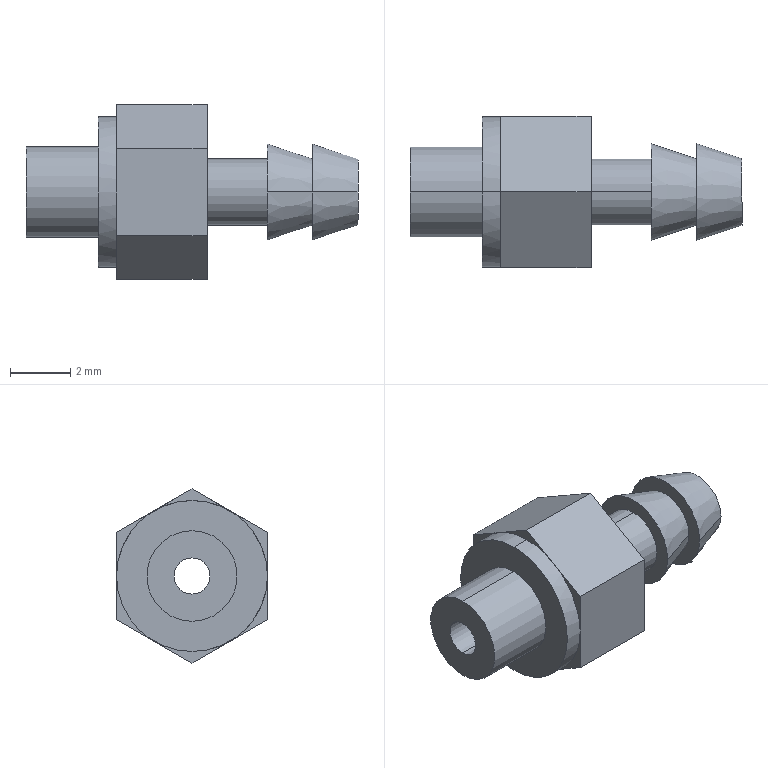Part | SolidWorks | features BaseBody 1 | 1 solid | 29 faces | box 11 x 5 x 5.774 mm | volume 106.233 mm3 | plane 17 | cylinder 8 | cone 4 | commonest cylinder face diameters 1.2 x2 2.2 x2 3 x2 5 x2
STEP:
#1=CARTESIAN_POINT('',(8.6,0.,-0.6));
#2=VERTEX_POINT('',#1);
#3=CARTESIAN_POINT('',(8.6,0.,0.6));
#4=VERTEX_POINT('',#3);
#5=CARTESIAN_POINT('',(8.6,0.,0.));
#6=DIRECTION('',(-1.,0.,0.));
#7=DIRECTION('',(0.,0.,1.));
#8=AXIS2_PLACEMENT_3D('',#5,#6,#7);
#9=CIRCLE('',#8,0.6);
#10=EDGE_CURVE('',#2,#4,#9,.T.);
#11=ORIENTED_EDGE('',*,*,#10,.F.);
#12=CARTESIAN_POINT('',(-2.4,0.,-0.6));
#13=VERTEX_POINT('',#12);
#14=CARTESIAN_POINT('',(-2.675,0.,-0.6));
#15=DIRECTION('',(-1.,0.,0.));
#16=VECTOR('',#15,1000.);
#17=LINE('',#14,#16);
#18=EDGE_CURVE('',#2,#13,#17,.T.);
#19=ORIENTED_EDGE('',*,*,#18,.T.);
#20=CARTESIAN_POINT('',(-2.4,0.,0.6));
#21=VERTEX_POINT('',#20);
#22=CARTESIAN_POINT('',(-2.4,0.,0.));
#23=DIRECTION('',(1.,0.,0.));
#24=DIRECTION('',(0.,0.,1.));
#25=AXIS2_PLACEMENT_3D('',#22,#23,#24);
#26=CIRCLE('',#25,0.6);
#27=EDGE_CURVE('',#21,#13,#26,.T.);
#28=ORIENTED_EDGE('',*,*,#27,.F.);
#29=CARTESIAN_POINT('',(-2.675,0.,0.6));
#30=DIRECTION('',(-1.,0.,0.));
#31=VECTOR('',#30,1000.);
#32=LINE('',#29,#31);
#33=EDGE_CURVE('',#4,#21,#32,.T.);
#34=ORIENTED_EDGE('',*,*,#33,.F.);
#35=EDGE_LOOP('',(#11,#19,#28,#34));
#36=FACE_OUTER_BOUND('',#35,.T.);
#37=CARTESIAN_POINT('',(-2.675,0.,0.));
#38=DIRECTION('',(-1.,0.,0.));
#39=DIRECTION('',(0.,0.,1.));
#40=AXIS2_PLACEMENT_3D('',#37,#38,#39);
#41=CYLINDRICAL_SURFACE('',#40,0.6);
#42=ADVANCED_FACE('',(#36),#41,.F.);
#43=CARTESIAN_POINT('',(8.6,-1.1,0.));
#44=VERTEX_POINT('',#43);
#45=CARTESIAN_POINT('',(8.6,1.1,0.));
#46=VERTEX_POINT('',#45);
#47=CARTESIAN_POINT('',(8.6,0.,0.));
#48=DIRECTION('',(-1.,0.,0.));
#49=DIRECTION('',(0.,-1.,0.));
#50=AXIS2_PLACEMENT_3D('',#47,#48,#49);
#51=CIRCLE('',#50,1.1);
#52=EDGE_CURVE('',#44,#46,#51,.T.);
#53=ORIENTED_EDGE('',*,*,#52,.T.);
#54=CARTESIAN_POINT('',(7.1,1.6,0.));
#55=VERTEX_POINT('',#54);
#56=CARTESIAN_POINT('',(7.1,1.6,0.));
#57=DIRECTION('',(-0.9487,0.3162,0.));
#58=VECTOR('',#57,1000.);
#59=LINE('',#56,#58);
#60=EDGE_CURVE('',#46,#55,#59,.T.);
#61=ORIENTED_EDGE('',*,*,#60,.T.);
#62=CARTESIAN_POINT('',(7.1,-1.6,0.));
#63=VERTEX_POINT('',#62);
#64=CARTESIAN_POINT('',(7.1,0.,0.));
#65=DIRECTION('',(1.,0.,0.));
#66=DIRECTION('',(0.,-1.,0.));
#67=AXIS2_PLACEMENT_3D('',#64,#65,#66);
#68=CIRCLE('',#67,1.6);
#69=EDGE_CURVE('',#55,#63,#68,.T.);
#70=ORIENTED_EDGE('',*,*,#69,.T.);
#71=CARTESIAN_POINT('',(7.1,-1.6,0.));
#72=DIRECTION('',(-0.9487,-0.3162,0.));
#73=VECTOR('',#72,1000.);
#74=LINE('',#71,#73);
#75=EDGE_CURVE('',#44,#63,#74,.T.);
#76=ORIENTED_EDGE('',*,*,#75,.F.);
#77=EDGE_LOOP('',(#53,#61,#70,#76));
#78=FACE_OUTER_BOUND('',#77,.T.);
#79=CARTESIAN_POINT('',(7.1,0.,0.));
#80=DIRECTION('',(-1.,0.,0.));
#81=DIRECTION('',(0.,-1.,0.));
#82=AXIS2_PLACEMENT_3D('',#79,#80,#81);
#83=CONICAL_SURFACE('',#82,1.6,0.3218);
#84=ADVANCED_FACE('',(#78),#83,.T.);
#85=CARTESIAN_POINT('',(-2.4,0.,-1.5));
#86=VERTEX_POINT('',#85);
#87=CARTESIAN_POINT('',(-2.4,0.,1.5));
#88=VERTEX_POINT('',#87);
#89=CARTESIAN_POINT('',(-2.4,0.,0.));
#90=DIRECTION('',(1.,0.,0.));
#91=DIRECTION('',(0.,0.,-1.));
#92=AXIS2_PLACEMENT_3D('',#89,#90,#91);
#93=CIRCLE('',#92,1.5);
#94=EDGE_CURVE('',#86,#88,#93,.T.);
#95=ORIENTED_EDGE('',*,*,#94,.T.);
#96=CARTESIAN_POINT('',(0.,0.,1.5));
#97=VERTEX_POINT('',#96);
#98=CARTESIAN_POINT('',(0.06,0.,1.5));
#99=DIRECTION('',(1.,0.,0.));
#100=VECTOR('',#99,1000.);
#101=LINE('',#98,#100);
#102=EDGE_CURVE('',#88,#97,#101,.T.);
#103=ORIENTED_EDGE('',*,*,#102,.T.);
#104=CARTESIAN_POINT('',(0.,0.,-1.5));
#105=VERTEX_POINT('',#104);
#106=CARTESIAN_POINT('',(0.,0.,0.));
#107=DIRECTION('',(-1.,0.,0.));
#108=DIRECTION('',(0.,0.,-1.));
#109=AXIS2_PLACEMENT_3D('',#106,#107,#108);
#110=CIRCLE('',#109,1.5);
#111=EDGE_CURVE('',#97,#105,#110,.T.);
#112=ORIENTED_EDGE('',*,*,#111,.T.);
#113=CARTESIAN_POINT('',(0.06,0.,-1.5));
#114=DIRECTION('',(1.,0.,0.));
#115=VECTOR('',#114,1000.);
#116=LINE('',#113,#115);
#117=EDGE_CURVE('',#86,#105,#116,.T.);
#118=ORIENTED_EDGE('',*,*,#117,.F.);
#119=EDGE_LOOP('',(#95,#103,#112,#118));
#120=FACE_OUTER_BOUND('',#119,.T.);
#121=CARTESIAN_POINT('',(0.06,0.,0.));
#122=DIRECTION('',(1.,0.,0.));
#123=DIRECTION('',(0.,0.,-1.));
#124=AXIS2_PLACEMENT_3D('',#121,#122,#123);
#125=CYLINDRICAL_SURFACE('',#124,1.5);
#126=ADVANCED_FACE('',(#120),#125,.T.);
#127=CARTESIAN_POINT('',(7.1,-1.1,0.));
#128=VERTEX_POINT('',#127);
#129=CARTESIAN_POINT('',(7.1,1.1,0.));
#130=VERTEX_POINT('',#129);
#131=CARTESIAN_POINT('',(7.1,0.,0.));
#132=DIRECTION('',(-1.,0.,0.));
#133=DIRECTION('',(0.,-1.,0.));
#134=AXIS2_PLACEMENT_3D('',#131,#132,#133);
#135=CIRCLE('',#134,1.1);
#136=EDGE_CURVE('',#128,#130,#135,.T.);
#137=ORIENTED_EDGE('',*,*,#136,.T.);
#138=CARTESIAN_POINT('',(5.6,1.6,0.));
#139=VERTEX_POINT('',#138);
#140=CARTESIAN_POINT('',(5.6,1.6,0.));
#141=DIRECTION('',(-0.9487,0.3162,0.));
#142=VECTOR('',#141,1000.);
#143=LINE('',#140,#142);
#144=EDGE_CURVE('',#130,#139,#143,.T.);
#145=ORIENTED_EDGE('',*,*,#144,.T.);
#146=CARTESIAN_POINT('',(5.6,-1.6,0.));
#147=VERTEX_POINT('',#146);
#148=CARTESIAN_POINT('',(5.6,0.,0.));
#149=DIRECTION('',(1.,0.,0.));
#150=DIRECTION('',(0.,-1.,0.));
#151=AXIS2_PLACEMENT_3D('',#148,#149,#150);
#152=CIRCLE('',#151,1.6);
#153=EDGE_CURVE('',#139,#147,#152,.T.);
#154=ORIENTED_EDGE('',*,*,#153,.T.);
#155=CARTESIAN_POINT('',(5.6,-1.6,0.));
#156=DIRECTION('',(-0.9487,-0.3162,0.));
#157=VECTOR('',#156,1000.);
#158=LINE('',#155,#157);
#159=EDGE_CURVE('',#128,#147,#158,.T.);
#160=ORIENTED_EDGE('',*,*,#159,.F.);
#161=EDGE_LOOP('',(#137,#145,#154,#160));
#162=FACE_OUTER_BOUND('',#161,.T.);
#163=CARTESIAN_POINT('',(5.6,0.,0.));
#164=DIRECTION('',(-1.,0.,0.));
#165=DIRECTION('',(0.,-1.,0.));
#166=AXIS2_PLACEMENT_3D('',#163,#164,#165);
#167=CONICAL_SURFACE('',#166,1.6,0.3218);
#168=ADVANCED_FACE('',(#162),#167,.T.);
#169=CARTESIAN_POINT('',(0.,0.,-2.5));
#170=VERTEX_POINT('',#169);
#171=CARTESIAN_POINT('',(0.,0.,2.5));
#172=VERTEX_POINT('',#171);
#173=CARTESIAN_POINT('',(0.,0.,0.));
#174=DIRECTION('',(1.,0.,0.));
#175=DIRECTION('',(0.,0.,-1.));
#176=AXIS2_PLACEMENT_3D('',#173,#174,#175);
#177=CIRCLE('',#176,2.5);
#178=EDGE_CURVE('',#170,#172,#177,.T.);
#179=ORIENTED_EDGE('',*,*,#178,.T.);
#180=CARTESIAN_POINT('',(0.6,0.,2.5));
#181=VERTEX_POINT('',#180);
#182=CARTESIAN_POINT('',(0.615,0.,2.5));
#183=DIRECTION('',(1.,0.,0.));
#184=VECTOR('',#183,1000.);
#185=LINE('',#182,#184);
#186=EDGE_CURVE('',#172,#181,#185,.T.);
#187=ORIENTED_EDGE('',*,*,#186,.T.);
#188=CARTESIAN_POINT('',(0.6,1.25,2.165));
#189=VERTEX_POINT('',#188);
#190=CARTESIAN_POINT('',(0.6,0.,0.));
#191=DIRECTION('',(-1.,0.,0.));
#192=DIRECTION('',(0.,0.,-1.));
#193=AXIS2_PLACEMENT_3D('',#190,#191,#192);
#194=CIRCLE('',#193,2.5);
#195=EDGE_CURVE('',#181,#189,#194,.T.);
#196=ORIENTED_EDGE('',*,*,#195,.T.);
#197=CARTESIAN_POINT('',(0.6,2.5,0.));
#198=VERTEX_POINT('',#197);
#199=CARTESIAN_POINT('',(0.6,0.,0.));
#200=DIRECTION('',(-1.,0.,0.));
#201=DIRECTION('',(0.,0.,-1.));
#202=AXIS2_PLACEMENT_3D('',#199,#200,#201);
#203=CIRCLE('',#202,2.5);
#204=EDGE_CURVE('',#189,#198,#203,.T.);
#205=ORIENTED_EDGE('',*,*,#204,.T.);
#206=CARTESIAN_POINT('',(0.6,0.,-2.5));
#207=VERTEX_POINT('',#206);
#208=CARTESIAN_POINT('',(0.6,0.,0.));
#209=DIRECTION('',(-1.,0.,0.));
#210=DIRECTION('',(0.,0.,-1.));
#211=AXIS2_PLACEMENT_3D('',#208,#209,#210);
#212=CIRCLE('',#211,2.5);
#213=EDGE_CURVE('',#198,#207,#212,.T.);
#214=ORIENTED_EDGE('',*,*,#213,.T.);
#215=CARTESIAN_POINT('',(0.615,0.,-2.5));
#216=DIRECTION('',(1.,0.,0.));
#217=VECTOR('',#216,1000.);
#218=LINE('',#215,#217);
#219=EDGE_CURVE('',#170,#207,#218,.T.);
#220=ORIENTED_EDGE('',*,*,#219,.F.);
#221=EDGE_LOOP('',(#179,#187,#196,#205,#214,#220));
#222=FACE_OUTER_BOUND('',#221,.T.);
#223=CARTESIAN_POINT('',(0.615,0.,0.));
#224=DIRECTION('',(1.,0.,0.));
#225=DIRECTION('',(0.,0.,-1.));
#226=AXIS2_PLACEMENT_3D('',#223,#224,#225);
#227=CYLINDRICAL_SURFACE('',#226,2.5);
#228=ADVANCED_FACE('',(#222),#227,.T.);
#229=CARTESIAN_POINT('',(3.6,0.,-1.1));
#230=VERTEX_POINT('',#229);
#231=CARTESIAN_POINT('',(3.6,0.,1.1));
#232=VERTEX_POINT('',#231);
#233=CARTESIAN_POINT('',(3.6,0.,0.));
#234=DIRECTION('',(1.,0.,0.));
#235=DIRECTION('',(0.,0.,-1.));
#236=AXIS2_PLACEMENT_3D('',#233,#234,#235);
#237=CIRCLE('',#236,1.1);
#238=EDGE_CURVE('',#230,#232,#237,.T.);
#239=ORIENTED_EDGE('',*,*,#238,.T.);
#240=CARTESIAN_POINT('',(5.6,0.,1.1));
#241=VERTEX_POINT('',#240);
#242=CARTESIAN_POINT('',(5.65,0.,1.1));
#243=DIRECTION('',(1.,0.,0.));
#244=VECTOR('',#243,1000.);
#245=LINE('',#242,#244);
#246=EDGE_CURVE('',#232,#241,#245,.T.);
#247=ORIENTED_EDGE('',*,*,#246,.T.);
#248=CARTESIAN_POINT('',(5.6,0.,-1.1));
#249=VERTEX_POINT('',#248);
#250=CARTESIAN_POINT('',(5.6,0.,0.));
#251=DIRECTION('',(-1.,0.,0.));
#252=DIRECTION('',(0.,0.,-1.));
#253=AXIS2_PLACEMENT_3D('',#250,#251,#252);
#254=CIRCLE('',#253,1.1);
#255=EDGE_CURVE('',#241,#249,#254,.T.);
#256=ORIENTED_EDGE('',*,*,#255,.T.);
#257=CARTESIAN_POINT('',(5.65,0.,-1.1));
#258=DIRECTION('',(1.,0.,0.));
#259=VECTOR('',#258,1000.);
#260=LINE('',#257,#259);
#261=EDGE_CURVE('',#230,#249,#260,.T.);
#262=ORIENTED_EDGE('',*,*,#261,.F.);
#263=EDGE_LOOP('',(#239,#247,#256,#262));
#264=FACE_OUTER_BOUND('',#263,.T.);
#265=CARTESIAN_POINT('',(5.65,0.,0.));
#266=DIRECTION('',(1.,0.,0.));
#267=DIRECTION('',(0.,0.,-1.));
#268=AXIS2_PLACEMENT_3D('',#265,#266,#267);
#269=CYLINDRICAL_SURFACE('',#268,1.1);
#270=ADVANCED_FACE('',(#264),#269,.T.);
#271=ORIENTED_EDGE('',*,*,#18,.F.);
#272=CARTESIAN_POINT('',(8.6,0.,0.));
#273=DIRECTION('',(-1.,0.,0.));
#274=DIRECTION('',(0.,0.,1.));
#275=AXIS2_PLACEMENT_3D('',#272,#273,#274);
#276=CIRCLE('',#275,0.6);
#277=EDGE_CURVE('',#4,#2,#276,.T.);
#278=ORIENTED_EDGE('',*,*,#277,.F.);
#279=ORIENTED_EDGE('',*,*,#33,.T.);
#280=CARTESIAN_POINT('',(-2.4,0.,0.));
#281=DIRECTION('',(1.,0.,0.));
#282=DIRECTION('',(0.,0.,1.));
#283=AXIS2_PLACEMENT_3D('',#280,#281,#282);
#284=CIRCLE('',#283,0.6);
#285=EDGE_CURVE('',#13,#21,#284,.T.);
#286=ORIENTED_EDGE('',*,*,#285,.F.);
#287=EDGE_LOOP('',(#271,#278,#279,#286));
#288=FACE_OUTER_BOUND('',#287,.T.);
#289=CARTESIAN_POINT('',(-2.675,0.,0.));
#290=DIRECTION('',(-1.,0.,0.));
#291=DIRECTION('',(0.,0.,1.));
#292=AXIS2_PLACEMENT_3D('',#289,#290,#291);
#293=CYLINDRICAL_SURFACE('',#292,0.6);
#294=ADVANCED_FACE('',(#288),#293,.F.);
#295=ORIENTED_EDGE('',*,*,#277,.T.);
#296=ORIENTED_EDGE('',*,*,#10,.T.);
#297=EDGE_LOOP('',(#295,#296));
#298=FACE_BOUND('',#297,.T.);
#299=ORIENTED_EDGE('',*,*,#52,.F.);
#300=CARTESIAN_POINT('',(8.6,0.,0.));
#301=DIRECTION('',(-1.,0.,0.));
#302=DIRECTION('',(0.,-1.,0.));
#303=AXIS2_PLACEMENT_3D('',#300,#301,#302);
#304=CIRCLE('',#303,1.1);
#305=EDGE_CURVE('',#46,#44,#304,.T.);
#306=ORIENTED_EDGE('',*,*,#305,.F.);
#307=EDGE_LOOP('',(#299,#306));
#308=FACE_OUTER_BOUND('',#307,.T.);
#309=CARTESIAN_POINT('',(8.6,-1.21,0.000000029));
#310=DIRECTION('',(-1.,0.,0.));
#311=DIRECTION('',(0.,0.,1.));
#312=AXIS2_PLACEMENT_3D('',#309,#310,#311);
#313=PLANE('',#312);
#314=ADVANCED_FACE('',(#298,#308),#313,.F.);
#315=ORIENTED_EDGE('',*,*,#27,.T.);
#316=ORIENTED_EDGE('',*,*,#285,.T.);
#317=EDGE_LOOP('',(#315,#316));
#318=FACE_BOUND('',#317,.T.);
#319=ORIENTED_EDGE('',*,*,#94,.F.);
#320=CARTESIAN_POINT('',(-2.4,0.,0.));
#321=DIRECTION('',(1.,0.,0.));
#322=DIRECTION('',(0.,0.,-1.));
#323=AXIS2_PLACEMENT_3D('',#320,#321,#322);
#324=CIRCLE('',#323,1.5);
#325=EDGE_CURVE('',#88,#86,#324,.T.);
#326=ORIENTED_EDGE('',*,*,#325,.F.);
#327=EDGE_LOOP('',(#319,#326));
#328=FACE_OUTER_BOUND('',#327,.T.);
#329=CARTESIAN_POINT('',(-2.4,-1.65,-0.00000004));
#330=DIRECTION('',(1.,0.,0.));
#331=DIRECTION('',(0.,0.,-1.));
#332=AXIS2_PLACEMENT_3D('',#329,#330,#331);
#333=PLANE('',#332);
#334=ADVANCED_FACE('',(#318,#328),#333,.F.);
#335=ORIENTED_EDGE('',*,*,#60,.F.);
#336=ORIENTED_EDGE('',*,*,#305,.T.);
#337=ORIENTED_EDGE('',*,*,#75,.T.);
#338=CARTESIAN_POINT('',(7.1,0.,0.));
#339=DIRECTION('',(1.,0.,0.));
#340=DIRECTION('',(0.,-1.,0.));
#341=AXIS2_PLACEMENT_3D('',#338,#339,#340);
#342=CIRCLE('',#341,1.6);
#343=EDGE_CURVE('',#63,#55,#342,.T.);
#344=ORIENTED_EDGE('',*,*,#343,.T.);
#345=EDGE_LOOP('',(#335,#336,#337,#344));
#346=FACE_OUTER_BOUND('',#345,.T.);
#347=CARTESIAN_POINT('',(7.1,0.,0.));
#348=DIRECTION('',(-1.,0.,0.));
#349=DIRECTION('',(0.,-1.,0.));
#350=AXIS2_PLACEMENT_3D('',#347,#348,#349);
#351=CONICAL_SURFACE('',#350,1.6,0.3218);
#352=ADVANCED_FACE('',(#346),#351,.T.);
#353=ORIENTED_EDGE('',*,*,#102,.F.);
#354=ORIENTED_EDGE('',*,*,#325,.T.);
#355=ORIENTED_EDGE('',*,*,#117,.T.);
#356=CARTESIAN_POINT('',(0.,0.,0.));
#357=DIRECTION('',(-1.,0.,0.));
#358=DIRECTION('',(0.,0.,-1.));
#359=AXIS2_PLACEMENT_3D('',#356,#357,#358);
#360=CIRCLE('',#359,1.5);
#361=EDGE_CURVE('',#105,#97,#360,.T.);
#362=ORIENTED_EDGE('',*,*,#361,.T.);
#363=EDGE_LOOP('',(#353,#354,#355,#362));
#364=FACE_OUTER_BOUND('',#363,.T.);
#365=CARTESIAN_POINT('',(0.06,0.,0.));
#366=DIRECTION('',(1.,0.,0.));
#367=DIRECTION('',(0.,0.,-1.));
#368=AXIS2_PLACEMENT_3D('',#365,#366,#367);
#369=CYLINDRICAL_SURFACE('',#368,1.5);
#370=ADVANCED_FACE('',(#364),#369,.T.);
#371=ORIENTED_EDGE('',*,*,#136,.F.);
#372=CARTESIAN_POINT('',(7.1,0.,0.));
#373=DIRECTION('',(-1.,0.,0.));
#374=DIRECTION('',(0.,-1.,0.));
#375=AXIS2_PLACEMENT_3D('',#372,#373,#374);
#376=CIRCLE('',#375,1.1);
#377=EDGE_CURVE('',#130,#128,#376,.T.);
#378=ORIENTED_EDGE('',*,*,#377,.F.);
#379=EDGE_LOOP('',(#371,#378));
#380=FACE_BOUND('',#379,.T.);
#381=ORIENTED_EDGE('',*,*,#343,.F.);
#382=ORIENTED_EDGE('',*,*,#69,.F.);
#383=EDGE_LOOP('',(#381,#382));
#384=FACE_OUTER_BOUND('',#383,.T.);
#385=CARTESIAN_POINT('',(7.1,-1.76,-0.000000043));
#386=DIRECTION('',(1.,0.,0.));
#387=DIRECTION('',(0.,0.,-1.));
#388=AXIS2_PLACEMENT_3D('',#385,#386,#387);
#389=PLANE('',#388);
#390=ADVANCED_FACE('',(#380,#384),#389,.F.);
#391=ORIENTED_EDGE('',*,*,#361,.F.);
#392=ORIENTED_EDGE('',*,*,#111,.F.);
#393=EDGE_LOOP('',(#391,#392));
#394=FACE_BOUND('',#393,.T.);
#395=ORIENTED_EDGE('',*,*,#178,.F.);
#396=CARTESIAN_POINT('',(0.,0.,0.));
#397=DIRECTION('',(1.,0.,0.));
#398=DIRECTION('',(0.,0.,-1.));
#399=AXIS2_PLACEMENT_3D('',#396,#397,#398);
#400=CIRCLE('',#399,2.5);
#401=EDGE_CURVE('',#172,#170,#400,.T.);
#402=ORIENTED_EDGE('',*,*,#401,.F.);
#403=EDGE_LOOP('',(#395,#402));
#404=FACE_OUTER_BOUND('',#403,.T.);
#405=CARTESIAN_POINT('',(0.,-2.75,-0.000000067));
#406=DIRECTION('',(1.,0.,0.));
#407=DIRECTION('',(0.,0.,-1.));
#408=AXIS2_PLACEMENT_3D('',#405,#406,#407);
#409=PLANE('',#408);
#410=ADVANCED_FACE('',(#394,#404),#409,.F.);
#411=ORIENTED_EDGE('',*,*,#144,.F.);
#412=ORIENTED_EDGE('',*,*,#377,.T.);
#413=ORIENTED_EDGE('',*,*,#159,.T.);
#414=CARTESIAN_POINT('',(5.6,0.,0.));
#415=DIRECTION('',(1.,0.,0.));
#416=DIRECTION('',(0.,-1.,0.));
#417=AXIS2_PLACEMENT_3D('',#414,#415,#416);
#418=CIRCLE('',#417,1.6);
#419=EDGE_CURVE('',#147,#139,#418,.T.);
#420=ORIENTED_EDGE('',*,*,#419,.T.);
#421=EDGE_LOOP('',(#411,#412,#413,#420));
#422=FACE_OUTER_BOUND('',#421,.T.);
#423=CARTESIAN_POINT('',(5.6,0.,0.));
#424=DIRECTION('',(-1.,0.,0.));
#425=DIRECTION('',(0.,-1.,0.));
#426=AXIS2_PLACEMENT_3D('',#423,#424,#425);
#427=CONICAL_SURFACE('',#426,1.6,0.3218);
#428=ADVANCED_FACE('',(#422),#427,.T.);
#429=ORIENTED_EDGE('',*,*,#186,.F.);
#430=ORIENTED_EDGE('',*,*,#401,.T.);
#431=ORIENTED_EDGE('',*,*,#219,.T.);
#432=CARTESIAN_POINT('',(0.6,-1.241,-2.17));
#433=VERTEX_POINT('',#432);
#434=CARTESIAN_POINT('',(0.6,0.,0.));
#435=DIRECTION('',(-1.,0.,0.));
#436=DIRECTION('',(0.,0.,-1.));
#437=AXIS2_PLACEMENT_3D('',#434,#435,#436);
#438=CIRCLE('',#437,2.5);
#439=EDGE_CURVE('',#207,#433,#438,.T.);
#440=ORIENTED_EDGE('',*,*,#439,.T.);
#441=CARTESIAN_POINT('',(0.6,-1.259,-2.16));
#442=VERTEX_POINT('',#441);
#443=CARTESIAN_POINT('',(0.6,-1.259,-2.16));
#444=CARTESIAN_POINT('',(0.6,-1.253,-2.163));
#445=CARTESIAN_POINT('',(0.6,-1.247,-2.167));
#446=CARTESIAN_POINT('',(0.6,-1.241,-2.17));
#447=B_SPLINE_CURVE_WITH_KNOTS('',3,(#443,#444,#445,#446),.UNSPECIFIED.,.F.,.F.,(4,4),(0.,1.),.UNSPECIFIED.);
#448=EDGE_CURVE('',#442,#433,#447,.T.);
#449=ORIENTED_EDGE('',*,*,#448,.F.);
#450=CARTESIAN_POINT('',(0.6,-2.5,0.));
#451=VERTEX_POINT('',#450);
#452=CARTESIAN_POINT('',(0.6,0.,0.));
#453=DIRECTION('',(-1.,0.,0.));
#454=DIRECTION('',(0.,0.,-1.));
#455=AXIS2_PLACEMENT_3D('',#452,#453,#454);
#456=CIRCLE('',#455,2.5);
#457=EDGE_CURVE('',#442,#451,#456,.T.);
#458=ORIENTED_EDGE('',*,*,#457,.T.);
#459=CARTESIAN_POINT('',(0.6,-1.25,2.165));
#460=VERTEX_POINT('',#459);
#461=CARTESIAN_POINT('',(0.6,0.,0.));
#462=DIRECTION('',(-1.,0.,0.));
#463=DIRECTION('',(0.,0.,-1.));
#464=AXIS2_PLACEMENT_3D('',#461,#462,#463);
#465=CIRCLE('',#464,2.5);
#466=EDGE_CURVE('',#451,#460,#465,.T.);
#467=ORIENTED_EDGE('',*,*,#466,.T.);
#468=CARTESIAN_POINT('',(0.6,0.,0.));
#469=DIRECTION('',(-1.,0.,0.));
#470=DIRECTION('',(0.,0.,-1.));
#471=AXIS2_PLACEMENT_3D('',#468,#469,#470);
#472=CIRCLE('',#471,2.5);
#473=EDGE_CURVE('',#460,#181,#472,.T.);
#474=ORIENTED_EDGE('',*,*,#473,.T.);
#475=EDGE_LOOP('',(#429,#430,#431,#440,#449,#458,#467,#474));
#476=FACE_OUTER_BOUND('',#475,.T.);
#477=CARTESIAN_POINT('',(0.615,0.,0.));
#478=DIRECTION('',(1.,0.,0.));
#479=DIRECTION('',(0.,0.,-1.));
#480=AXIS2_PLACEMENT_3D('',#477,#478,#479);
#481=CYLINDRICAL_SURFACE('',#480,2.5);
#482=ADVANCED_FACE('',(#476),#481,.T.);
#483=CARTESIAN_POINT('',(5.6,0.,0.));
#484=DIRECTION('',(-1.,0.,0.));
#485=DIRECTION('',(0.,0.,-1.));
#486=AXIS2_PLACEMENT_3D('',#483,#484,#485);
#487=CIRCLE('',#486,1.1);
#488=EDGE_CURVE('',#249,#241,#487,.T.);
#489=ORIENTED_EDGE('',*,*,#488,.F.);
#490=ORIENTED_EDGE('',*,*,#255,.F.);
#491=EDGE_LOOP('',(#489,#490));
#492=FACE_BOUND('',#491,.T.);
#493=ORIENTED_EDGE('',*,*,#419,.F.);
#494=ORIENTED_EDGE('',*,*,#153,.F.);
#495=EDGE_LOOP('',(#493,#494));
#496=FACE_OUTER_BOUND('',#495,.T.);
#497=CARTESIAN_POINT('',(5.6,-1.76,-0.000000043));
#498=DIRECTION('',(1.,0.,0.));
#499=DIRECTION('',(0.,0.,-1.));
#500=AXIS2_PLACEMENT_3D('',#497,#498,#499);
#501=PLANE('',#500);
#502=ADVANCED_FACE('',(#492,#496),#501,.F.);
#503=CARTESIAN_POINT('',(0.6,2.5,1.443));
#504=VERTEX_POINT('',#503);
#505=CARTESIAN_POINT('',(0.6,1.25,2.165));
#506=DIRECTION('',(0.,-0.866,0.5));
#507=VECTOR('',#506,1000.);
#508=LINE('',#505,#507);
#509=EDGE_CURVE('',#504,#189,#508,.T.);
#510=ORIENTED_EDGE('',*,*,#509,.F.);
#511=CARTESIAN_POINT('',(0.6,2.5,-0.00002883));
#512=DIRECTION('',(0.,0.,1.));
#513=VECTOR('',#512,1000.);
#514=LINE('',#511,#513);
#515=EDGE_CURVE('',#198,#504,#514,.T.);
#516=ORIENTED_EDGE('',*,*,#515,.F.);
#517=ORIENTED_EDGE('',*,*,#204,.F.);
#518=EDGE_LOOP('',(#510,#516,#517));
#519=FACE_OUTER_BOUND('',#518,.T.);
#520=CARTESIAN_POINT('',(0.6,1.875,-0.1081));
#521=DIRECTION('',(1.,0.,0.));
#522=DIRECTION('',(0.,0.,-1.));
#523=AXIS2_PLACEMENT_3D('',#520,#521,#522);
#524=PLANE('',#523);
#525=ADVANCED_FACE('',(#519),#524,.F.);
#526=CARTESIAN_POINT('',(0.6,0.,2.887));
#527=VERTEX_POINT('',#526);
#528=CARTESIAN_POINT('',(0.6,-1.25,2.165));
#529=DIRECTION('',(0.,-0.866,-0.5));
#530=VECTOR('',#529,1000.);
#531=LINE('',#528,#530);
#532=EDGE_CURVE('',#527,#460,#531,.T.);
#533=ORIENTED_EDGE('',*,*,#532,.F.);
#534=CARTESIAN_POINT('',(0.6,1.25,2.165));
#535=DIRECTION('',(0.,-0.866,0.5));
#536=VECTOR('',#535,1000.);
#537=LINE('',#534,#536);
#538=EDGE_CURVE('',#189,#527,#537,.T.);
#539=ORIENTED_EDGE('',*,*,#538,.F.);
#540=ORIENTED_EDGE('',*,*,#195,.F.);
#541=ORIENTED_EDGE('',*,*,#473,.F.);
#542=EDGE_LOOP('',(#533,#539,#540,#541));
#543=FACE_OUTER_BOUND('',#542,.T.);
#544=CARTESIAN_POINT('',(0.6,-0.000002132,2.129));
#545=DIRECTION('',(1.,0.,0.));
#546=DIRECTION('',(0.,0.,-1.));
#547=AXIS2_PLACEMENT_3D('',#544,#545,#546);
#548=PLANE('',#547);
#549=ADVANCED_FACE('',(#543),#548,.F.);
#550=CARTESIAN_POINT('',(0.6,-2.5,1.443));
#551=VERTEX_POINT('',#550);
#552=CARTESIAN_POINT('',(0.6,-2.5,0.00002383));
#553=DIRECTION('',(0.,0.,-1.));
#554=VECTOR('',#553,1000.);
#555=LINE('',#552,#554);
#556=EDGE_CURVE('',#551,#451,#555,.T.);
#557=ORIENTED_EDGE('',*,*,#556,.F.);
#558=CARTESIAN_POINT('',(0.6,-1.25,2.165));
#559=DIRECTION('',(0.,-0.866,-0.5));
#560=VECTOR('',#559,1000.);
#561=LINE('',#558,#560);
#562=EDGE_CURVE('',#460,#551,#561,.T.);
#563=ORIENTED_EDGE('',*,*,#562,.F.);
#564=ORIENTED_EDGE('',*,*,#466,.F.);
#565=EDGE_LOOP('',(#557,#563,#564));
#566=FACE_OUTER_BOUND('',#565,.T.);
#567=CARTESIAN_POINT('',(0.6,-1.875,-0.1081));
#568=DIRECTION('',(1.,0.,0.));
#569=DIRECTION('',(0.,0.,-1.));
#570=AXIS2_PLACEMENT_3D('',#567,#568,#569);
#571=PLANE('',#570);
#572=ADVANCED_FACE('',(#566),#571,.F.);
#573=CARTESIAN_POINT('',(0.6,-2.5,-1.443));
#574=VERTEX_POINT('',#573);
#575=CARTESIAN_POINT('',(0.6,-1.25,-2.165));
#576=DIRECTION('',(0.,0.866,-0.5));
#577=VECTOR('',#576,1000.);
#578=LINE('',#575,#577);
#579=EDGE_CURVE('',#574,#442,#578,.T.);
#580=ORIENTED_EDGE('',*,*,#579,.F.);
#581=CARTESIAN_POINT('',(0.6,-2.5,0.00002383));
#582=DIRECTION('',(0.,0.,-1.));
#583=VECTOR('',#582,1000.);
#584=LINE('',#581,#583);
#585=EDGE_CURVE('',#451,#574,#584,.T.);
#586=ORIENTED_EDGE('',*,*,#585,.F.);
#587=ORIENTED_EDGE('',*,*,#457,.F.);
#588=EDGE_LOOP('',(#580,#586,#587));
#589=FACE_OUTER_BOUND('',#588,.T.);
#590=CARTESIAN_POINT('',(0.6,-1.88,-2.267));
#591=DIRECTION('',(1.,0.,0.));
#592=DIRECTION('',(0.,0.,-1.));
#593=AXIS2_PLACEMENT_3D('',#590,#591,#592);
#594=PLANE('',#593);
#595=ADVANCED_FACE('',(#589),#594,.F.);
#596=CARTESIAN_POINT('',(0.6,2.5,-1.443));
#597=VERTEX_POINT('',#596);
#598=CARTESIAN_POINT('',(0.6,2.5,-0.00002883));
#599=DIRECTION('',(0.,0.,1.));
#600=VECTOR('',#599,1000.);
#601=LINE('',#598,#600);
#602=EDGE_CURVE('',#597,#198,#601,.T.);
#603=ORIENTED_EDGE('',*,*,#602,.F.);
#604=CARTESIAN_POINT('',(0.6,0.00005,-2.887));
#605=VERTEX_POINT('',#604);
#606=CARTESIAN_POINT('',(0.6,0.00005,-2.887));
#607=DIRECTION('',(0.,0.866,0.5));
#608=VECTOR('',#607,1000.);
#609=LINE('',#606,#608);
#610=EDGE_CURVE('',#605,#597,#609,.T.);
#611=ORIENTED_EDGE('',*,*,#610,.F.);
#612=CARTESIAN_POINT('',(0.6,-1.25,-2.165));
#613=DIRECTION('',(0.,0.866,-0.5));
#614=VECTOR('',#613,1000.);
#615=LINE('',#612,#614);
#616=EDGE_CURVE('',#433,#605,#615,.T.);
#617=ORIENTED_EDGE('',*,*,#616,.F.);
#618=ORIENTED_EDGE('',*,*,#439,.F.);
#619=ORIENTED_EDGE('',*,*,#213,.F.);
#620=EDGE_LOOP('',(#603,#611,#617,#618,#619));
#621=FACE_OUTER_BOUND('',#620,.T.);
#622=CARTESIAN_POINT('',(0.6,0.6297,-3.031));
#623=DIRECTION('',(1.,0.,0.));
#624=DIRECTION('',(0.,0.,-1.));
#625=AXIS2_PLACEMENT_3D('',#622,#623,#624);
#626=PLANE('',#625);
#627=ADVANCED_FACE('',(#621),#626,.F.);
#628=ORIENTED_EDGE('',*,*,#246,.F.);
#629=CARTESIAN_POINT('',(3.6,0.,0.));
#630=DIRECTION('',(1.,0.,0.));
#631=DIRECTION('',(0.,0.,-1.));
#632=AXIS2_PLACEMENT_3D('',#629,#630,#631);
#633=CIRCLE('',#632,1.1);
#634=EDGE_CURVE('',#232,#230,#633,.T.);
#635=ORIENTED_EDGE('',*,*,#634,.T.);
#636=ORIENTED_EDGE('',*,*,#261,.T.);
#637=ORIENTED_EDGE('',*,*,#488,.T.);
#638=EDGE_LOOP('',(#628,#635,#636,#637));
#639=FACE_OUTER_BOUND('',#638,.T.);
#640=CARTESIAN_POINT('',(5.65,0.,0.));
#641=DIRECTION('',(1.,0.,0.));
#642=DIRECTION('',(0.,0.,-1.));
#643=AXIS2_PLACEMENT_3D('',#640,#641,#642);
#644=CYLINDRICAL_SURFACE('',#643,1.1);
#645=ADVANCED_FACE('',(#639),#644,.T.);
#646=CARTESIAN_POINT('',(3.6,2.5,-1.443));
#647=VERTEX_POINT('',#646);
#648=CARTESIAN_POINT('',(3.6,0.00005,-2.887));
#649=VERTEX_POINT('',#648);
#650=CARTESIAN_POINT('',(3.6,1.25,-2.165));
#651=DIRECTION('',(0.,-0.866,-0.5));
#652=VECTOR('',#651,1000.);
#653=LINE('',#650,#652);
#654=EDGE_CURVE('',#647,#649,#653,.T.);
#655=ORIENTED_EDGE('',*,*,#654,.T.);
#656=CARTESIAN_POINT('',(0.4502,0.00005,-2.887));
#657=DIRECTION('',(-1.,0.,0.));
#658=VECTOR('',#657,1000.);
#659=LINE('',#656,#658);
#660=EDGE_CURVE('',#649,#605,#659,.T.);
#661=ORIENTED_EDGE('',*,*,#660,.T.);
#662=ORIENTED_EDGE('',*,*,#610,.T.);
#663=CARTESIAN_POINT('',(0.4502,2.5,-1.443));
#664=DIRECTION('',(1.,0.,0.));
#665=VECTOR('',#664,1000.);
#666=LINE('',#663,#665);
#667=EDGE_CURVE('',#597,#647,#666,.T.);
#668=ORIENTED_EDGE('',*,*,#667,.T.);
#669=EDGE_LOOP('',(#655,#661,#662,#668));
#670=FACE_OUTER_BOUND('',#669,.T.);
#671=CARTESIAN_POINT('',(0.4502,1.25,-2.165));
#672=DIRECTION('',(0.,0.5,-0.866));
#673=DIRECTION('',(0.,0.866,0.5));
#674=AXIS2_PLACEMENT_3D('',#671,#672,#673);
#675=PLANE('',#674);
#676=ADVANCED_FACE('',(#670),#675,.T.);
#677=ORIENTED_EDGE('',*,*,#238,.F.);
#678=ORIENTED_EDGE('',*,*,#634,.F.);
#679=EDGE_LOOP('',(#677,#678));
#680=FACE_BOUND('',#679,.T.);
#681=CARTESIAN_POINT('',(3.6,2.5,1.443));
#682=VERTEX_POINT('',#681);
#683=CARTESIAN_POINT('',(3.6,0.,2.887));
#684=VERTEX_POINT('',#683);
#685=CARTESIAN_POINT('',(3.6,2.5,1.443));
#686=DIRECTION('',(0.,-0.866,0.5));
#687=VECTOR('',#686,1000.);
#688=LINE('',#685,#687);
#689=EDGE_CURVE('',#682,#684,#688,.T.);
#690=ORIENTED_EDGE('',*,*,#689,.T.);
#691=CARTESIAN_POINT('',(3.6,-2.5,1.443));
#692=VERTEX_POINT('',#691);
#693=CARTESIAN_POINT('',(3.6,0.,2.887));
#694=DIRECTION('',(0.,-0.866,-0.5));
#695=VECTOR('',#694,1000.);
#696=LINE('',#693,#695);
#697=EDGE_CURVE('',#684,#692,#696,.T.);
#698=ORIENTED_EDGE('',*,*,#697,.T.);
#699=CARTESIAN_POINT('',(3.6,-2.5,-1.443));
#700=VERTEX_POINT('',#699);
#701=CARTESIAN_POINT('',(3.6,-2.5,-3.175));
#702=DIRECTION('',(0.,0.,-1.));
#703=VECTOR('',#702,1000.);
#704=LINE('',#701,#703);
#705=EDGE_CURVE('',#692,#700,#704,.T.);
#706=ORIENTED_EDGE('',*,*,#705,.T.);
#707=CARTESIAN_POINT('',(3.6,-2.5,-1.443));
#708=DIRECTION('',(0.,0.866,-0.5));
#709=VECTOR('',#708,1000.);
#710=LINE('',#707,#709);
#711=EDGE_CURVE('',#700,#649,#710,.T.);
#712=ORIENTED_EDGE('',*,*,#711,.T.);
#713=ORIENTED_EDGE('',*,*,#654,.F.);
#714=CARTESIAN_POINT('',(3.6,2.5,-3.175));
#715=DIRECTION('',(0.,0.,1.));
#716=VECTOR('',#715,1000.);
#717=LINE('',#714,#716);
#718=EDGE_CURVE('',#647,#682,#717,.T.);
#719=ORIENTED_EDGE('',*,*,#718,.T.);
#720=EDGE_LOOP('',(#690,#698,#706,#712,#713,#719));
#721=FACE_OUTER_BOUND('',#720,.T.);
#722=CARTESIAN_POINT('',(3.6,0.000000067,-3.175));
#723=DIRECTION('',(1.,0.,0.));
#724=DIRECTION('',(0.,0.,-1.));
#725=AXIS2_PLACEMENT_3D('',#722,#723,#724);
#726=PLANE('',#725);
#727=ADVANCED_FACE('',(#680,#721),#726,.T.);
#728=ORIENTED_EDGE('',*,*,#579,.T.);
#729=ORIENTED_EDGE('',*,*,#448,.T.);
#730=ORIENTED_EDGE('',*,*,#616,.T.);
#731=ORIENTED_EDGE('',*,*,#660,.F.);
#732=ORIENTED_EDGE('',*,*,#711,.F.);
#733=CARTESIAN_POINT('',(0.4502,-2.5,-1.443));
#734=DIRECTION('',(-1.,0.,0.));
#735=VECTOR('',#734,1000.);
#736=LINE('',#733,#735);
#737=EDGE_CURVE('',#700,#574,#736,.T.);
#738=ORIENTED_EDGE('',*,*,#737,.T.);
#739=EDGE_LOOP('',(#728,#729,#730,#731,#732,#738));
#740=FACE_OUTER_BOUND('',#739,.T.);
#741=CARTESIAN_POINT('',(0.4502,-1.25,-2.165));
#742=DIRECTION('',(0.,-0.5,-0.866));
#743=DIRECTION('',(0.,0.866,-0.5));
#744=AXIS2_PLACEMENT_3D('',#741,#742,#743);
#745=PLANE('',#744);
#746=ADVANCED_FACE('',(#740),#745,.T.);
#747=ORIENTED_EDGE('',*,*,#667,.F.);
#748=ORIENTED_EDGE('',*,*,#602,.T.);
#749=ORIENTED_EDGE('',*,*,#515,.T.);
#750=CARTESIAN_POINT('',(0.4502,2.5,1.443));
#751=DIRECTION('',(1.,0.,0.));
#752=VECTOR('',#751,1000.);
#753=LINE('',#750,#752);
#754=EDGE_CURVE('',#504,#682,#753,.T.);
#755=ORIENTED_EDGE('',*,*,#754,.T.);
#756=ORIENTED_EDGE('',*,*,#718,.F.);
#757=EDGE_LOOP('',(#747,#748,#749,#755,#756));
#758=FACE_OUTER_BOUND('',#757,.T.);
#759=CARTESIAN_POINT('',(0.4502,2.5,-0.00002883));
#760=DIRECTION('',(0.,1.,0.));
#761=DIRECTION('',(0.,0.,1.));
#762=AXIS2_PLACEMENT_3D('',#759,#760,#761);
#763=PLANE('',#762);
#764=ADVANCED_FACE('',(#758),#763,.T.);
#765=CARTESIAN_POINT('',(0.4502,0.,2.887));
#766=DIRECTION('',(-1.,0.,0.));
#767=VECTOR('',#766,1000.);
#768=LINE('',#765,#767);
#769=EDGE_CURVE('',#684,#527,#768,.T.);
#770=ORIENTED_EDGE('',*,*,#769,.T.);
#771=ORIENTED_EDGE('',*,*,#532,.T.);
#772=ORIENTED_EDGE('',*,*,#562,.T.);
#773=CARTESIAN_POINT('',(0.4502,-2.5,1.443));
#774=DIRECTION('',(1.,0.,0.));
#775=VECTOR('',#774,1000.);
#776=LINE('',#773,#775);
#777=EDGE_CURVE('',#551,#692,#776,.T.);
#778=ORIENTED_EDGE('',*,*,#777,.T.);
#779=ORIENTED_EDGE('',*,*,#697,.F.);
#780=EDGE_LOOP('',(#770,#771,#772,#778,#779));
#781=FACE_OUTER_BOUND('',#780,.T.);
#782=CARTESIAN_POINT('',(0.4502,-1.25,2.165));
#783=DIRECTION('',(0.,-0.5,0.866));
#784=DIRECTION('',(0.,-0.866,-0.5));
#785=AXIS2_PLACEMENT_3D('',#782,#783,#784);
#786=PLANE('',#785);
#787=ADVANCED_FACE('',(#781),#786,.T.);
#788=ORIENTED_EDGE('',*,*,#754,.F.);
#789=ORIENTED_EDGE('',*,*,#509,.T.);
#790=ORIENTED_EDGE('',*,*,#538,.T.);
#791=ORIENTED_EDGE('',*,*,#769,.F.);
#792=ORIENTED_EDGE('',*,*,#689,.F.);
#793=EDGE_LOOP('',(#788,#789,#790,#791,#792));
#794=FACE_OUTER_BOUND('',#793,.T.);
#795=CARTESIAN_POINT('',(0.4502,1.25,2.165));
#796=DIRECTION('',(0.,0.5,0.866));
#797=DIRECTION('',(0.,-0.866,0.5));
#798=AXIS2_PLACEMENT_3D('',#795,#796,#797);
#799=PLANE('',#798);
#800=ADVANCED_FACE('',(#794),#799,.T.);
#801=ORIENTED_EDGE('',*,*,#777,.F.);
#802=ORIENTED_EDGE('',*,*,#556,.T.);
#803=ORIENTED_EDGE('',*,*,#585,.T.);
#804=ORIENTED_EDGE('',*,*,#737,.F.);
#805=ORIENTED_EDGE('',*,*,#705,.F.);
#806=EDGE_LOOP('',(#801,#802,#803,#804,#805));
#807=FACE_OUTER_BOUND('',#806,.T.);
#808=CARTESIAN_POINT('',(0.4502,-2.5,0.00002383));
#809=DIRECTION('',(0.,-1.,0.));
#810=DIRECTION('',(0.,0.,-1.));
#811=AXIS2_PLACEMENT_3D('',#808,#809,#810);
#812=PLANE('',#811);
#813=ADVANCED_FACE('',(#807),#812,.T.);
#814=CLOSED_SHELL('',(#42,#84,#126,#168,#228,#270,#294,#314,#334,#352,#370,#390,#410,#428,#482,#502,#525,#549,#572,#595,#627,#645,#676,#727,#746,#764,#787,#800,#813));
#815=MANIFOLD_SOLID_BREP('',#814);
#816=CARTESIAN_POINT('',(0.,0.,0.));
#817=DIRECTION('',(0.,0.,1.));
#818=DIRECTION('',(1.,0.,0.));
#819=AXIS2_PLACEMENT_3D('',#816,#817,#818);
#820=(LENGTH_UNIT()NAMED_UNIT(*)SI_UNIT(.MILLI.,.METRE.));
#821=UNCERTAINTY_MEASURE_WITH_UNIT(LENGTH_MEASURE(0.00001),#820,'','');
#822=(NAMED_UNIT(*)PLANE_ANGLE_UNIT()SI_UNIT($,.RADIAN.));
#823=(NAMED_UNIT(*)SI_UNIT($,.STERADIAN.)SOLID_ANGLE_UNIT());
#824=(GEOMETRIC_REPRESENTATION_CONTEXT(3)GLOBAL_UNCERTAINTY_ASSIGNED_CONTEXT((#821))GLOBAL_UNIT_ASSIGNED_CONTEXT((#820,#822,#823))REPRESENTATION_CONTEXT('',''));
#825=ADVANCED_BREP_SHAPE_REPRESENTATION('',(#815,#819),#824);